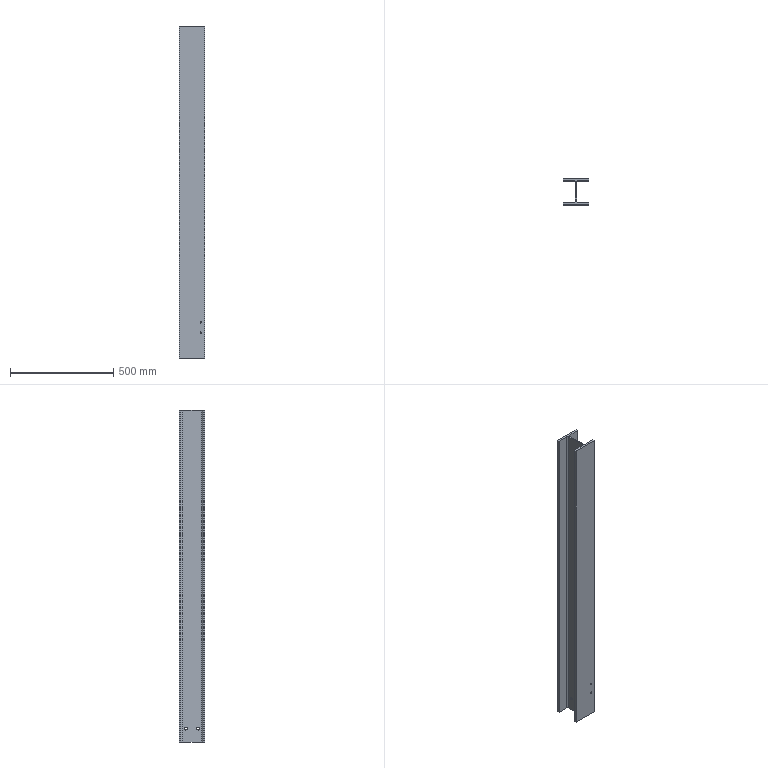Part | STEP file | 01-H125X125X6.5X9_default<machining> | 1 solid | 30 faces | box 125 x 125 x 1610 mm | volume 4827397 mm3 | cylinder 16 | plane 14 | commonest cylinder face diameters 6.8 x8 14 x4 16 x4